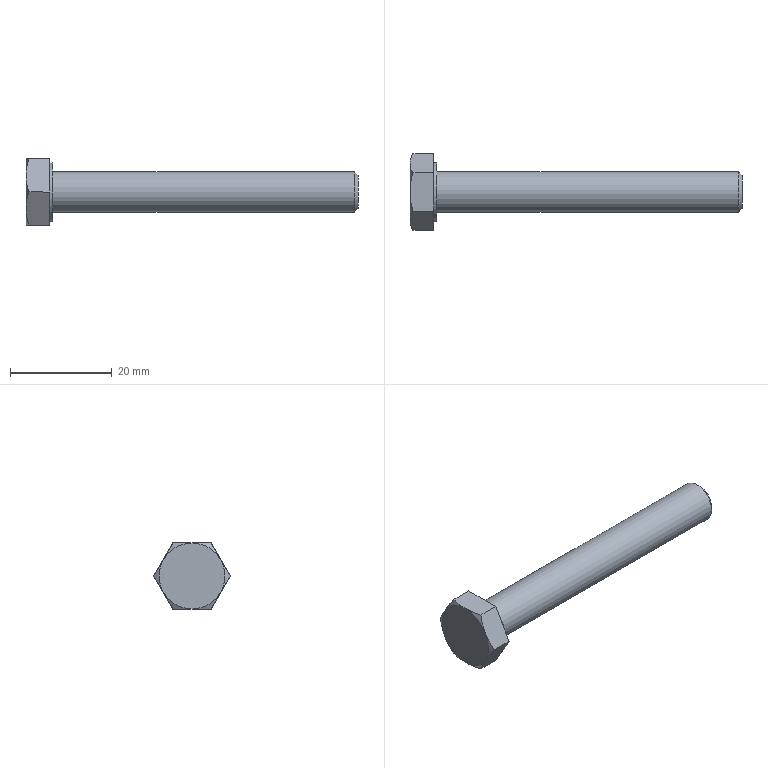Part | STEP file | DIN 931-1 - M8 x 60 | 1 solid | 19 faces | box 65.3 x 15.011 x 13 mm | volume 3758 mm3 | plane 10 | cone 7 | cylinder 2 | commonest cylinder face diameters 8 x1 11.6 x1